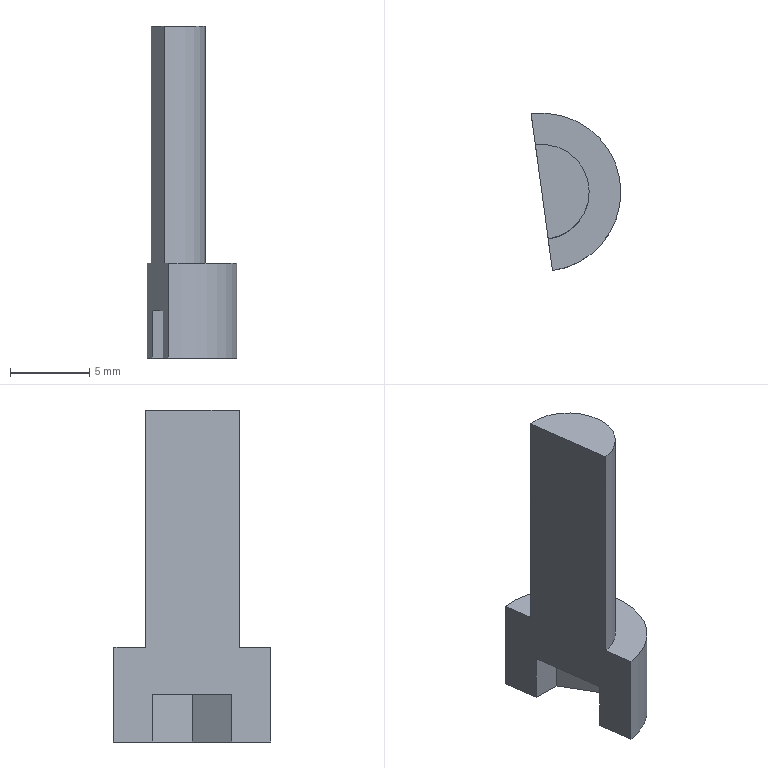Part | STEP file | LG M6_1.5F | 1 solid | 12 faces | box 5.673 x 9.954 x 21 mm | volume 414.941 mm3 | plane 9 | cylinder 3 | commonest cylinder face diameters 10 x2 6 x1
STEP:
#1=CARTESIAN_POINT('',(0.,0.,0.));
#2=DIRECTION('',(0.,0.,1.));
#3=DIRECTION('',(1.,0.,0.));
#4=AXIS2_PLACEMENT_3D('',#1,#2,#3);
#5=CARTESIAN_POINT('',(0.6731,-4.954,-6.));
#6=VERTEX_POINT('',#5);
#7=CARTESIAN_POINT('',(5.,0.,-6.));
#8=VERTEX_POINT('',#7);
#9=CARTESIAN_POINT('',(0.,0.,-6.));
#10=DIRECTION('',(0.,0.,1.));
#11=DIRECTION('',(1.,0.,0.));
#12=AXIS2_PLACEMENT_3D('',#9,#10,#11);
#13=CIRCLE('',#12,5.);
#14=CARTESIAN_POINT('',(0.,0.,-6.));
#15=DIRECTION('',(0.,0.,1.));
#16=DIRECTION('',(1.,0.,0.));
#17=AXIS2_PLACEMENT_3D('',#14,#15,#16);
#18=CYLINDRICAL_SURFACE('',#17,5.);
#19=CARTESIAN_POINT('',(0.,0.));
#20=DIRECTION('',(1.,0.));
#21=VECTOR('',#20,1.);
#22=LINE('',#19,#21);
#23=(GEOMETRIC_REPRESENTATION_CONTEXT(2)PARAMETRIC_REPRESENTATION_CONTEXT()REPRESENTATION_CONTEXT('',''));
#24=DEFINITIONAL_REPRESENTATION('',(#22),#23);
#25=PCURVE('',#18,#24);
#26=CARTESIAN_POINT('',(0.,0.,-6.));
#27=DIRECTION('',(0.,0.,1.));
#28=DIRECTION('',(1.,0.,0.));
#29=AXIS2_PLACEMENT_3D('',#26,#27,#28);
#30=PLANE('',#29);
#31=CARTESIAN_POINT('',(0.,0.));
#32=DIRECTION('',(1.,0.));
#33=AXIS2_PLACEMENT_2D('',#31,#32);
#34=CIRCLE('',#33,5.);
#35=(GEOMETRIC_REPRESENTATION_CONTEXT(2)PARAMETRIC_REPRESENTATION_CONTEXT()REPRESENTATION_CONTEXT('',''));
#36=DEFINITIONAL_REPRESENTATION('',(#34),#35);
#37=PCURVE('',#30,#36);
#38=SURFACE_CURVE('',#13,(#25,#37),.PCURVE_S1.);
#39=EDGE_CURVE('',#6,#8,#38,.T.);
#40=ORIENTED_EDGE('',*,*,#39,.T.);
#41=CARTESIAN_POINT('',(5.,0.,0.));
#42=VERTEX_POINT('',#41);
#43=CARTESIAN_POINT('',(5.,0.,-6.));
#44=DIRECTION('',(0.,0.,1.));
#45=VECTOR('',#44,1.);
#46=LINE('',#43,#45);
#47=CARTESIAN_POINT('',(6.283,0.));
#48=DIRECTION('',(0.,1.));
#49=VECTOR('',#48,1.);
#50=LINE('',#47,#49);
#51=(GEOMETRIC_REPRESENTATION_CONTEXT(2)PARAMETRIC_REPRESENTATION_CONTEXT()REPRESENTATION_CONTEXT('',''));
#52=DEFINITIONAL_REPRESENTATION('',(#50),#51);
#53=PCURVE('',#18,#52);
#54=CARTESIAN_POINT('',(0.,0.,-6.));
#55=DIRECTION('',(0.,0.,1.));
#56=DIRECTION('',(1.,0.,0.));
#57=AXIS2_PLACEMENT_3D('',#54,#55,#56);
#58=CYLINDRICAL_SURFACE('',#57,5.);
#59=CARTESIAN_POINT('',(0.,0.));
#60=DIRECTION('',(0.,1.));
#61=VECTOR('',#60,1.);
#62=LINE('',#59,#61);
#63=(GEOMETRIC_REPRESENTATION_CONTEXT(2)PARAMETRIC_REPRESENTATION_CONTEXT()REPRESENTATION_CONTEXT('',''));
#64=DEFINITIONAL_REPRESENTATION('',(#62),#63);
#65=PCURVE('',#58,#64);
#66=SURFACE_CURVE('',#46,(#53,#65),.PCURVE_S1.);
#67=EDGE_CURVE('',#8,#42,#66,.T.);
#68=ORIENTED_EDGE('',*,*,#67,.T.);
#69=CARTESIAN_POINT('',(0.6731,-4.954,0.));
#70=VERTEX_POINT('',#69);
#71=CARTESIAN_POINT('',(0.,0.,0.));
#72=DIRECTION('',(0.,0.,1.));
#73=DIRECTION('',(1.,0.,0.));
#74=AXIS2_PLACEMENT_3D('',#71,#72,#73);
#75=CIRCLE('',#74,5.);
#76=CARTESIAN_POINT('',(0.,6.));
#77=DIRECTION('',(1.,0.));
#78=VECTOR('',#77,1.);
#79=LINE('',#76,#78);
#80=(GEOMETRIC_REPRESENTATION_CONTEXT(2)PARAMETRIC_REPRESENTATION_CONTEXT()REPRESENTATION_CONTEXT('',''));
#81=DEFINITIONAL_REPRESENTATION('',(#79),#80);
#82=PCURVE('',#18,#81);
#83=CARTESIAN_POINT('',(0.,0.,0.));
#84=DIRECTION('',(0.,0.,1.));
#85=DIRECTION('',(1.,0.,0.));
#86=AXIS2_PLACEMENT_3D('',#83,#84,#85);
#87=PLANE('',#86);
#88=CARTESIAN_POINT('',(0.,0.));
#89=DIRECTION('',(1.,0.));
#90=AXIS2_PLACEMENT_2D('',#88,#89);
#91=CIRCLE('',#90,5.);
#92=(GEOMETRIC_REPRESENTATION_CONTEXT(2)PARAMETRIC_REPRESENTATION_CONTEXT()REPRESENTATION_CONTEXT('',''));
#93=DEFINITIONAL_REPRESENTATION('',(#91),#92);
#94=PCURVE('',#87,#93);
#95=SURFACE_CURVE('',#75,(#82,#94),.PCURVE_S1.);
#96=EDGE_CURVE('',#70,#42,#95,.T.);
#97=ORIENTED_EDGE('',*,*,#96,.F.);
#98=CARTESIAN_POINT('',(0.6731,-4.954,-6.));
#99=DIRECTION('',(0.,0.,1.));
#100=VECTOR('',#99,1.);
#101=LINE('',#98,#100);
#102=CARTESIAN_POINT('',(4.847,0.));
#103=DIRECTION('',(0.,1.));
#104=VECTOR('',#103,1.);
#105=LINE('',#102,#104);
#106=(GEOMETRIC_REPRESENTATION_CONTEXT(2)PARAMETRIC_REPRESENTATION_CONTEXT()REPRESENTATION_CONTEXT('',''));
#107=DEFINITIONAL_REPRESENTATION('',(#105),#106);
#108=PCURVE('',#18,#107);
#109=CARTESIAN_POINT('',(8.077,-59.454,72.57));
#110=DIRECTION('',(0.9909,0.1346,0.));
#111=DIRECTION('',(0.1346,-0.9909,0.));
#112=AXIS2_PLACEMENT_3D('',#109,#110,#111);
#113=PLANE('',#112);
#114=CARTESIAN_POINT('',(-55.,78.57));
#115=DIRECTION('',(0.,-1.));
#116=VECTOR('',#115,1.);
#117=LINE('',#114,#116);
#118=(GEOMETRIC_REPRESENTATION_CONTEXT(2)PARAMETRIC_REPRESENTATION_CONTEXT()REPRESENTATION_CONTEXT('',''));
#119=DEFINITIONAL_REPRESENTATION('',(#117),#118);
#120=PCURVE('',#113,#119);
#121=SURFACE_CURVE('',#101,(#108,#120),.PCURVE_S1.);
#122=EDGE_CURVE('',#6,#70,#121,.T.);
#123=ORIENTED_EDGE('',*,*,#122,.F.);
#124=EDGE_LOOP('',(#40,#68,#97,#123));
#125=FACE_BOUND('',#124,.T.);
#126=ADVANCED_FACE('',(#125),#18,.T.);
#127=CARTESIAN_POINT('',(0.4039,-2.973,0.));
#128=VERTEX_POINT('',#127);
#129=CARTESIAN_POINT('',(0.,0.,0.));
#130=DIRECTION('',(-0.1346,0.9909,0.));
#131=VECTOR('',#130,1.);
#132=LINE('',#129,#131);
#133=CARTESIAN_POINT('',(0.,0.));
#134=DIRECTION('',(-0.1346,0.9909));
#135=VECTOR('',#134,1.);
#136=LINE('',#133,#135);
#137=(GEOMETRIC_REPRESENTATION_CONTEXT(2)PARAMETRIC_REPRESENTATION_CONTEXT()REPRESENTATION_CONTEXT('',''));
#138=DEFINITIONAL_REPRESENTATION('',(#136),#137);
#139=PCURVE('',#87,#138);
#140=CARTESIAN_POINT('',(-60.,72.57));
#141=DIRECTION('',(-1.,0.));
#142=VECTOR('',#141,1.);
#143=LINE('',#140,#142);
#144=(GEOMETRIC_REPRESENTATION_CONTEXT(2)PARAMETRIC_REPRESENTATION_CONTEXT()REPRESENTATION_CONTEXT('',''));
#145=DEFINITIONAL_REPRESENTATION('',(#143),#144);
#146=PCURVE('',#113,#145);
#147=SURFACE_CURVE('',#132,(#139,#146),.PCURVE_S1.);
#148=EDGE_CURVE('',#70,#128,#147,.T.);
#149=ORIENTED_EDGE('',*,*,#148,.F.);
#150=ORIENTED_EDGE('',*,*,#96,.T.);
#151=CARTESIAN_POINT('',(-0.6731,4.954,0.));
#152=VERTEX_POINT('',#151);
#153=CARTESIAN_POINT('',(0.,0.,0.));
#154=DIRECTION('',(0.,0.,1.));
#155=DIRECTION('',(1.,0.,0.));
#156=AXIS2_PLACEMENT_3D('',#153,#154,#155);
#157=CIRCLE('',#156,5.);
#158=CARTESIAN_POINT('',(0.,0.));
#159=DIRECTION('',(1.,0.));
#160=AXIS2_PLACEMENT_2D('',#158,#159);
#161=CIRCLE('',#160,5.);
#162=(GEOMETRIC_REPRESENTATION_CONTEXT(2)PARAMETRIC_REPRESENTATION_CONTEXT()REPRESENTATION_CONTEXT('',''));
#163=DEFINITIONAL_REPRESENTATION('',(#161),#162);
#164=PCURVE('',#87,#163);
#165=CARTESIAN_POINT('',(0.,6.));
#166=DIRECTION('',(1.,0.));
#167=VECTOR('',#166,1.);
#168=LINE('',#165,#167);
#169=(GEOMETRIC_REPRESENTATION_CONTEXT(2)PARAMETRIC_REPRESENTATION_CONTEXT()REPRESENTATION_CONTEXT('',''));
#170=DEFINITIONAL_REPRESENTATION('',(#168),#169);
#171=PCURVE('',#58,#170);
#172=SURFACE_CURVE('',#157,(#164,#171),.PCURVE_S1.);
#173=EDGE_CURVE('',#42,#152,#172,.T.);
#174=ORIENTED_EDGE('',*,*,#173,.T.);
#175=CARTESIAN_POINT('',(-0.4039,2.973,0.));
#176=VERTEX_POINT('',#175);
#177=CARTESIAN_POINT('',(0.,0.,0.));
#178=DIRECTION('',(-0.1346,0.9909,0.));
#179=VECTOR('',#178,1.);
#180=LINE('',#177,#179);
#181=CARTESIAN_POINT('',(0.,0.));
#182=DIRECTION('',(-0.1346,0.9909));
#183=VECTOR('',#182,1.);
#184=LINE('',#181,#183);
#185=(GEOMETRIC_REPRESENTATION_CONTEXT(2)PARAMETRIC_REPRESENTATION_CONTEXT()REPRESENTATION_CONTEXT('',''));
#186=DEFINITIONAL_REPRESENTATION('',(#184),#185);
#187=PCURVE('',#87,#186);
#188=CARTESIAN_POINT('',(-60.,72.57));
#189=DIRECTION('',(-1.,0.));
#190=VECTOR('',#189,1.);
#191=LINE('',#188,#190);
#192=(GEOMETRIC_REPRESENTATION_CONTEXT(2)PARAMETRIC_REPRESENTATION_CONTEXT()REPRESENTATION_CONTEXT('',''));
#193=DEFINITIONAL_REPRESENTATION('',(#191),#192);
#194=PCURVE('',#113,#193);
#195=SURFACE_CURVE('',#180,(#187,#194),.PCURVE_S1.);
#196=EDGE_CURVE('',#176,#152,#195,.T.);
#197=ORIENTED_EDGE('',*,*,#196,.F.);
#198=CARTESIAN_POINT('',(0.,0.,0.));
#199=DIRECTION('',(0.,0.,1.));
#200=DIRECTION('',(1.,0.,0.));
#201=AXIS2_PLACEMENT_3D('',#198,#199,#200);
#202=CIRCLE('',#201,3.);
#203=CARTESIAN_POINT('',(0.,0.));
#204=DIRECTION('',(1.,0.));
#205=AXIS2_PLACEMENT_2D('',#203,#204);
#206=CIRCLE('',#205,3.);
#207=(GEOMETRIC_REPRESENTATION_CONTEXT(2)PARAMETRIC_REPRESENTATION_CONTEXT()REPRESENTATION_CONTEXT('',''));
#208=DEFINITIONAL_REPRESENTATION('',(#206),#207);
#209=PCURVE('',#87,#208);
#210=CARTESIAN_POINT('',(0.,0.,15.));
#211=DIRECTION('',(0.,0.,-1.));
#212=DIRECTION('',(-1.,0.,0.));
#213=AXIS2_PLACEMENT_3D('',#210,#211,#212);
#214=CYLINDRICAL_SURFACE('',#213,3.);
#215=CARTESIAN_POINT('',(9.425,15.));
#216=DIRECTION('',(-1.,0.));
#217=VECTOR('',#216,1.);
#218=LINE('',#215,#217);
#219=(GEOMETRIC_REPRESENTATION_CONTEXT(2)PARAMETRIC_REPRESENTATION_CONTEXT()REPRESENTATION_CONTEXT('',''));
#220=DEFINITIONAL_REPRESENTATION('',(#218),#219);
#221=PCURVE('',#214,#220);
#222=SURFACE_CURVE('',#202,(#209,#221),.PCURVE_S1.);
#223=EDGE_CURVE('',#128,#176,#222,.T.);
#224=ORIENTED_EDGE('',*,*,#223,.F.);
#225=EDGE_LOOP('',(#149,#150,#174,#197,#224));
#226=FACE_BOUND('',#225,.T.);
#227=ADVANCED_FACE('',(#226),#87,.T.);
#228=ORIENTED_EDGE('',*,*,#67,.F.);
#229=CARTESIAN_POINT('',(-0.6731,4.954,-6.));
#230=VERTEX_POINT('',#229);
#231=CARTESIAN_POINT('',(0.,0.,-6.));
#232=DIRECTION('',(0.,0.,1.));
#233=DIRECTION('',(1.,0.,0.));
#234=AXIS2_PLACEMENT_3D('',#231,#232,#233);
#235=CIRCLE('',#234,5.);
#236=CARTESIAN_POINT('',(0.,0.));
#237=DIRECTION('',(1.,0.));
#238=VECTOR('',#237,1.);
#239=LINE('',#236,#238);
#240=(GEOMETRIC_REPRESENTATION_CONTEXT(2)PARAMETRIC_REPRESENTATION_CONTEXT()REPRESENTATION_CONTEXT('',''));
#241=DEFINITIONAL_REPRESENTATION('',(#239),#240);
#242=PCURVE('',#58,#241);
#243=CARTESIAN_POINT('',(0.,0.));
#244=DIRECTION('',(1.,0.));
#245=AXIS2_PLACEMENT_2D('',#243,#244);
#246=CIRCLE('',#245,5.);
#247=(GEOMETRIC_REPRESENTATION_CONTEXT(2)PARAMETRIC_REPRESENTATION_CONTEXT()REPRESENTATION_CONTEXT('',''));
#248=DEFINITIONAL_REPRESENTATION('',(#246),#247);
#249=PCURVE('',#30,#248);
#250=SURFACE_CURVE('',#235,(#242,#249),.PCURVE_S1.);
#251=EDGE_CURVE('',#8,#230,#250,.T.);
#252=ORIENTED_EDGE('',*,*,#251,.T.);
#253=CARTESIAN_POINT('',(-0.6731,4.954,-6.));
#254=DIRECTION('',(0.,0.,-1.));
#255=VECTOR('',#254,1.);
#256=LINE('',#253,#255);
#257=CARTESIAN_POINT('',(1.706,0.));
#258=DIRECTION('',(0.,-1.));
#259=VECTOR('',#258,1.);
#260=LINE('',#257,#259);
#261=(GEOMETRIC_REPRESENTATION_CONTEXT(2)PARAMETRIC_REPRESENTATION_CONTEXT()REPRESENTATION_CONTEXT('',''));
#262=DEFINITIONAL_REPRESENTATION('',(#260),#261);
#263=PCURVE('',#58,#262);
#264=CARTESIAN_POINT('',(-65.,78.57));
#265=DIRECTION('',(0.,1.));
#266=VECTOR('',#265,1.);
#267=LINE('',#264,#266);
#268=(GEOMETRIC_REPRESENTATION_CONTEXT(2)PARAMETRIC_REPRESENTATION_CONTEXT()REPRESENTATION_CONTEXT('',''));
#269=DEFINITIONAL_REPRESENTATION('',(#267),#268);
#270=PCURVE('',#113,#269);
#271=SURFACE_CURVE('',#256,(#263,#270),.PCURVE_S1.);
#272=EDGE_CURVE('',#152,#230,#271,.T.);
#273=ORIENTED_EDGE('',*,*,#272,.F.);
#274=ORIENTED_EDGE('',*,*,#173,.F.);
#275=EDGE_LOOP('',(#228,#252,#273,#274));
#276=FACE_BOUND('',#275,.T.);
#277=ADVANCED_FACE('',(#276),#58,.T.);
#278=ORIENTED_EDGE('',*,*,#39,.F.);
#279=CARTESIAN_POINT('',(0.341,-2.51,-6.));
#280=VERTEX_POINT('',#279);
#281=CARTESIAN_POINT('',(0.,0.,-6.));
#282=DIRECTION('',(-0.1346,0.9909,0.));
#283=VECTOR('',#282,1.);
#284=LINE('',#281,#283);
#285=CARTESIAN_POINT('',(0.,0.));
#286=DIRECTION('',(-0.1346,0.9909));
#287=VECTOR('',#286,1.);
#288=LINE('',#285,#287);
#289=(GEOMETRIC_REPRESENTATION_CONTEXT(2)PARAMETRIC_REPRESENTATION_CONTEXT()REPRESENTATION_CONTEXT('',''));
#290=DEFINITIONAL_REPRESENTATION('',(#288),#289);
#291=PCURVE('',#30,#290);
#292=CARTESIAN_POINT('',(-60.,78.57));
#293=DIRECTION('',(-1.,0.));
#294=VECTOR('',#293,1.);
#295=LINE('',#292,#294);
#296=(GEOMETRIC_REPRESENTATION_CONTEXT(2)PARAMETRIC_REPRESENTATION_CONTEXT()REPRESENTATION_CONTEXT('',''));
#297=DEFINITIONAL_REPRESENTATION('',(#295),#296);
#298=PCURVE('',#113,#297);
#299=SURFACE_CURVE('',#284,(#291,#298),.PCURVE_S1.);
#300=EDGE_CURVE('',#6,#280,#299,.T.);
#301=ORIENTED_EDGE('',*,*,#300,.T.);
#302=CARTESIAN_POINT('',(1.449,-2.51,-6.));
#303=VERTEX_POINT('',#302);
#304=CARTESIAN_POINT('',(1.449,-2.51,-6.));
#305=DIRECTION('',(-1.,0.,0.));
#306=VECTOR('',#305,1.);
#307=LINE('',#304,#306);
#308=CARTESIAN_POINT('',(1.449,-2.51));
#309=DIRECTION('',(-1.,0.));
#310=VECTOR('',#309,1.);
#311=LINE('',#308,#310);
#312=(GEOMETRIC_REPRESENTATION_CONTEXT(2)PARAMETRIC_REPRESENTATION_CONTEXT()REPRESENTATION_CONTEXT('',''));
#313=DEFINITIONAL_REPRESENTATION('',(#311),#312);
#314=PCURVE('',#30,#313);
#315=CARTESIAN_POINT('',(1.449,-2.51,-3.));
#316=DIRECTION('',(0.,-1.,0.));
#317=DIRECTION('',(0.,0.,-1.));
#318=AXIS2_PLACEMENT_3D('',#315,#316,#317);
#319=PLANE('',#318);
#320=CARTESIAN_POINT('',(3.,0.));
#321=DIRECTION('',(0.,-1.));
#322=VECTOR('',#321,1.);
#323=LINE('',#320,#322);
#324=(GEOMETRIC_REPRESENTATION_CONTEXT(2)PARAMETRIC_REPRESENTATION_CONTEXT()REPRESENTATION_CONTEXT('',''));
#325=DEFINITIONAL_REPRESENTATION('',(#323),#324);
#326=PCURVE('',#319,#325);
#327=SURFACE_CURVE('',#307,(#314,#326),.PCURVE_S1.);
#328=EDGE_CURVE('',#303,#280,#327,.T.);
#329=ORIENTED_EDGE('',*,*,#328,.F.);
#330=CARTESIAN_POINT('',(2.898,0.,-6.));
#331=VERTEX_POINT('',#330);
#332=CARTESIAN_POINT('',(2.898,0.,-6.));
#333=DIRECTION('',(-0.5,-0.866,0.));
#334=VECTOR('',#333,1.);
#335=LINE('',#332,#334);
#336=CARTESIAN_POINT('',(2.898,0.));
#337=DIRECTION('',(-0.5,-0.866));
#338=VECTOR('',#337,1.);
#339=LINE('',#336,#338);
#340=(GEOMETRIC_REPRESENTATION_CONTEXT(2)PARAMETRIC_REPRESENTATION_CONTEXT()REPRESENTATION_CONTEXT('',''));
#341=DEFINITIONAL_REPRESENTATION('',(#339),#340);
#342=PCURVE('',#30,#341);
#343=CARTESIAN_POINT('',(2.898,0.,-3.));
#344=DIRECTION('',(0.866,-0.5,0.));
#345=DIRECTION('',(0.5,0.866,0.));
#346=AXIS2_PLACEMENT_3D('',#343,#344,#345);
#347=PLANE('',#346);
#348=CARTESIAN_POINT('',(0.,-3.));
#349=DIRECTION('',(-1.,0.));
#350=VECTOR('',#349,1.);
#351=LINE('',#348,#350);
#352=(GEOMETRIC_REPRESENTATION_CONTEXT(2)PARAMETRIC_REPRESENTATION_CONTEXT()REPRESENTATION_CONTEXT('',''));
#353=DEFINITIONAL_REPRESENTATION('',(#351),#352);
#354=PCURVE('',#347,#353);
#355=SURFACE_CURVE('',#335,(#342,#354),.PCURVE_S1.);
#356=EDGE_CURVE('',#331,#303,#355,.T.);
#357=ORIENTED_EDGE('',*,*,#356,.F.);
#358=CARTESIAN_POINT('',(1.449,2.51,-6.));
#359=VERTEX_POINT('',#358);
#360=CARTESIAN_POINT('',(1.449,2.51,-6.));
#361=DIRECTION('',(0.5,-0.866,0.));
#362=VECTOR('',#361,1.);
#363=LINE('',#360,#362);
#364=CARTESIAN_POINT('',(1.449,2.51));
#365=DIRECTION('',(0.5,-0.866));
#366=VECTOR('',#365,1.);
#367=LINE('',#364,#366);
#368=(GEOMETRIC_REPRESENTATION_CONTEXT(2)PARAMETRIC_REPRESENTATION_CONTEXT()REPRESENTATION_CONTEXT('',''));
#369=DEFINITIONAL_REPRESENTATION('',(#367),#368);
#370=PCURVE('',#30,#369);
#371=CARTESIAN_POINT('',(1.449,2.51,-3.));
#372=DIRECTION('',(0.866,0.5,0.));
#373=DIRECTION('',(-0.5,0.866,0.));
#374=AXIS2_PLACEMENT_3D('',#371,#372,#373);
#375=PLANE('',#374);
#376=CARTESIAN_POINT('',(0.,-3.));
#377=DIRECTION('',(-1.,0.));
#378=VECTOR('',#377,1.);
#379=LINE('',#376,#378);
#380=(GEOMETRIC_REPRESENTATION_CONTEXT(2)PARAMETRIC_REPRESENTATION_CONTEXT()REPRESENTATION_CONTEXT('',''));
#381=DEFINITIONAL_REPRESENTATION('',(#379),#380);
#382=PCURVE('',#375,#381);
#383=SURFACE_CURVE('',#363,(#370,#382),.PCURVE_S1.);
#384=EDGE_CURVE('',#359,#331,#383,.T.);
#385=ORIENTED_EDGE('',*,*,#384,.F.);
#386=CARTESIAN_POINT('',(-0.341,2.51,-6.));
#387=VERTEX_POINT('',#386);
#388=CARTESIAN_POINT('',(-1.449,2.51,-6.));
#389=DIRECTION('',(1.,0.,0.));
#390=VECTOR('',#389,1.);
#391=LINE('',#388,#390);
#392=CARTESIAN_POINT('',(-1.449,2.51));
#393=DIRECTION('',(1.,0.));
#394=VECTOR('',#393,1.);
#395=LINE('',#392,#394);
#396=(GEOMETRIC_REPRESENTATION_CONTEXT(2)PARAMETRIC_REPRESENTATION_CONTEXT()REPRESENTATION_CONTEXT('',''));
#397=DEFINITIONAL_REPRESENTATION('',(#395),#396);
#398=PCURVE('',#30,#397);
#399=CARTESIAN_POINT('',(-1.449,2.51,-3.));
#400=DIRECTION('',(0.,1.,0.));
#401=DIRECTION('',(0.,0.,1.));
#402=AXIS2_PLACEMENT_3D('',#399,#400,#401);
#403=PLANE('',#402);
#404=CARTESIAN_POINT('',(-3.,0.));
#405=DIRECTION('',(0.,1.));
#406=VECTOR('',#405,1.);
#407=LINE('',#404,#406);
#408=(GEOMETRIC_REPRESENTATION_CONTEXT(2)PARAMETRIC_REPRESENTATION_CONTEXT()REPRESENTATION_CONTEXT('',''));
#409=DEFINITIONAL_REPRESENTATION('',(#407),#408);
#410=PCURVE('',#403,#409);
#411=SURFACE_CURVE('',#391,(#398,#410),.PCURVE_S1.);
#412=EDGE_CURVE('',#387,#359,#411,.T.);
#413=ORIENTED_EDGE('',*,*,#412,.F.);
#414=CARTESIAN_POINT('',(0.,0.,-6.));
#415=DIRECTION('',(-0.1346,0.9909,0.));
#416=VECTOR('',#415,1.);
#417=LINE('',#414,#416);
#418=CARTESIAN_POINT('',(0.,0.));
#419=DIRECTION('',(-0.1346,0.9909));
#420=VECTOR('',#419,1.);
#421=LINE('',#418,#420);
#422=(GEOMETRIC_REPRESENTATION_CONTEXT(2)PARAMETRIC_REPRESENTATION_CONTEXT()REPRESENTATION_CONTEXT('',''));
#423=DEFINITIONAL_REPRESENTATION('',(#421),#422);
#424=PCURVE('',#30,#423);
#425=CARTESIAN_POINT('',(-60.,78.57));
#426=DIRECTION('',(-1.,0.));
#427=VECTOR('',#426,1.);
#428=LINE('',#425,#427);
#429=(GEOMETRIC_REPRESENTATION_CONTEXT(2)PARAMETRIC_REPRESENTATION_CONTEXT()REPRESENTATION_CONTEXT('',''));
#430=DEFINITIONAL_REPRESENTATION('',(#428),#429);
#431=PCURVE('',#113,#430);
#432=SURFACE_CURVE('',#417,(#424,#431),.PCURVE_S1.);
#433=EDGE_CURVE('',#387,#230,#432,.T.);
#434=ORIENTED_EDGE('',*,*,#433,.T.);
#435=ORIENTED_EDGE('',*,*,#251,.F.);
#436=EDGE_LOOP('',(#278,#301,#329,#357,#385,#413,#434,#435));
#437=FACE_BOUND('',#436,.T.);
#438=ADVANCED_FACE('',(#437),#30,.F.);
#439=CARTESIAN_POINT('',(0.4039,-2.973,15.));
#440=VERTEX_POINT('',#439);
#441=CARTESIAN_POINT('',(-0.4039,2.973,15.));
#442=VERTEX_POINT('',#441);
#443=CARTESIAN_POINT('',(0.,0.,15.));
#444=DIRECTION('',(0.,0.,1.));
#445=DIRECTION('',(1.,0.,0.));
#446=AXIS2_PLACEMENT_3D('',#443,#444,#445);
#447=CIRCLE('',#446,3.);
#448=CARTESIAN_POINT('',(9.425,0.));
#449=DIRECTION('',(-1.,0.));
#450=VECTOR('',#449,1.);
#451=LINE('',#448,#450);
#452=(GEOMETRIC_REPRESENTATION_CONTEXT(2)PARAMETRIC_REPRESENTATION_CONTEXT()REPRESENTATION_CONTEXT('',''));
#453=DEFINITIONAL_REPRESENTATION('',(#451),#452);
#454=PCURVE('',#214,#453);
#455=CARTESIAN_POINT('',(0.,0.,15.));
#456=DIRECTION('',(0.,0.,1.));
#457=DIRECTION('',(1.,0.,0.));
#458=AXIS2_PLACEMENT_3D('',#455,#456,#457);
#459=PLANE('',#458);
#460=CARTESIAN_POINT('',(0.,0.));
#461=DIRECTION('',(1.,0.));
#462=AXIS2_PLACEMENT_2D('',#460,#461);
#463=CIRCLE('',#462,3.);
#464=(GEOMETRIC_REPRESENTATION_CONTEXT(2)PARAMETRIC_REPRESENTATION_CONTEXT()REPRESENTATION_CONTEXT('',''));
#465=DEFINITIONAL_REPRESENTATION('',(#463),#464);
#466=PCURVE('',#459,#465);
#467=SURFACE_CURVE('',#447,(#454,#466),.PCURVE_S1.);
#468=EDGE_CURVE('',#440,#442,#467,.T.);
#469=ORIENTED_EDGE('',*,*,#468,.F.);
#470=CARTESIAN_POINT('',(0.4039,-2.973,15.));
#471=DIRECTION('',(0.,0.,-1.));
#472=VECTOR('',#471,1.);
#473=LINE('',#470,#472);
#474=CARTESIAN_POINT('',(4.577,0.));
#475=DIRECTION('',(0.,1.));
#476=VECTOR('',#475,1.);
#477=LINE('',#474,#476);
#478=(GEOMETRIC_REPRESENTATION_CONTEXT(2)PARAMETRIC_REPRESENTATION_CONTEXT()REPRESENTATION_CONTEXT('',''));
#479=DEFINITIONAL_REPRESENTATION('',(#477),#478);
#480=PCURVE('',#214,#479);
#481=CARTESIAN_POINT('',(-57.,57.57));
#482=DIRECTION('',(0.,1.));
#483=VECTOR('',#482,1.);
#484=LINE('',#481,#483);
#485=(GEOMETRIC_REPRESENTATION_CONTEXT(2)PARAMETRIC_REPRESENTATION_CONTEXT()REPRESENTATION_CONTEXT('',''));
#486=DEFINITIONAL_REPRESENTATION('',(#484),#485);
#487=PCURVE('',#113,#486);
#488=SURFACE_CURVE('',#473,(#480,#487),.PCURVE_S1.);
#489=EDGE_CURVE('',#440,#128,#488,.T.);
#490=ORIENTED_EDGE('',*,*,#489,.T.);
#491=ORIENTED_EDGE('',*,*,#223,.T.);
#492=CARTESIAN_POINT('',(-0.4039,2.973,15.));
#493=DIRECTION('',(0.,0.,1.));
#494=VECTOR('',#493,1.);
#495=LINE('',#492,#494);
#496=CARTESIAN_POINT('',(1.436,0.));
#497=DIRECTION('',(0.,-1.));
#498=VECTOR('',#497,1.);
#499=LINE('',#496,#498);
#500=(GEOMETRIC_REPRESENTATION_CONTEXT(2)PARAMETRIC_REPRESENTATION_CONTEXT()REPRESENTATION_CONTEXT('',''));
#501=DEFINITIONAL_REPRESENTATION('',(#499),#500);
#502=PCURVE('',#214,#501);
#503=CARTESIAN_POINT('',(-63.,57.57));
#504=DIRECTION('',(0.,-1.));
#505=VECTOR('',#504,1.);
#506=LINE('',#503,#505);
#507=(GEOMETRIC_REPRESENTATION_CONTEXT(2)PARAMETRIC_REPRESENTATION_CONTEXT()REPRESENTATION_CONTEXT('',''));
#508=DEFINITIONAL_REPRESENTATION('',(#506),#507);
#509=PCURVE('',#113,#508);
#510=SURFACE_CURVE('',#495,(#502,#509),.PCURVE_S1.);
#511=EDGE_CURVE('',#176,#442,#510,.T.);
#512=ORIENTED_EDGE('',*,*,#511,.T.);
#513=EDGE_LOOP('',(#469,#490,#491,#512));
#514=FACE_BOUND('',#513,.T.);
#515=ADVANCED_FACE('',(#514),#214,.T.);
#516=CARTESIAN_POINT('',(0.,0.,15.));
#517=DIRECTION('',(-0.1346,0.9909,0.));
#518=VECTOR('',#517,1.);
#519=LINE('',#516,#518);
#520=CARTESIAN_POINT('',(0.,0.));
#521=DIRECTION('',(-0.1346,0.9909));
#522=VECTOR('',#521,1.);
#523=LINE('',#520,#522);
#524=(GEOMETRIC_REPRESENTATION_CONTEXT(2)PARAMETRIC_REPRESENTATION_CONTEXT()REPRESENTATION_CONTEXT('',''));
#525=DEFINITIONAL_REPRESENTATION('',(#523),#524);
#526=PCURVE('',#459,#525);
#527=CARTESIAN_POINT('',(-60.,57.57));
#528=DIRECTION('',(-1.,0.));
#529=VECTOR('',#528,1.);
#530=LINE('',#527,#529);
#531=(GEOMETRIC_REPRESENTATION_CONTEXT(2)PARAMETRIC_REPRESENTATION_CONTEXT()REPRESENTATION_CONTEXT('',''));
#532=DEFINITIONAL_REPRESENTATION('',(#530),#531);
#533=PCURVE('',#113,#532);
#534=SURFACE_CURVE('',#519,(#526,#533),.PCURVE_S1.);
#535=EDGE_CURVE('',#440,#442,#534,.T.);
#536=ORIENTED_EDGE('',*,*,#535,.F.);
#537=ORIENTED_EDGE('',*,*,#468,.T.);
#538=EDGE_LOOP('',(#536,#537));
#539=FACE_BOUND('',#538,.T.);
#540=ADVANCED_FACE('',(#539),#459,.T.);
#541=ORIENTED_EDGE('',*,*,#328,.T.);
#542=CARTESIAN_POINT('',(0.341,-2.51,-3.));
#543=VERTEX_POINT('',#542);
#544=CARTESIAN_POINT('',(0.341,-2.51,-3.));
#545=DIRECTION('',(0.,0.,1.));
#546=VECTOR('',#545,1.);
#547=LINE('',#544,#546);
#548=CARTESIAN_POINT('',(0.,-1.108));
#549=DIRECTION('',(-1.,0.));
#550=VECTOR('',#549,1.);
#551=LINE('',#548,#550);
#552=(GEOMETRIC_REPRESENTATION_CONTEXT(2)PARAMETRIC_REPRESENTATION_CONTEXT()REPRESENTATION_CONTEXT('',''));
#553=DEFINITIONAL_REPRESENTATION('',(#551),#552);
#554=PCURVE('',#319,#553);
#555=CARTESIAN_POINT('',(-57.467,75.57));
#556=DIRECTION('',(0.,-1.));
#557=VECTOR('',#556,1.);
#558=LINE('',#555,#557);
#559=(GEOMETRIC_REPRESENTATION_CONTEXT(2)PARAMETRIC_REPRESENTATION_CONTEXT()REPRESENTATION_CONTEXT('',''));
#560=DEFINITIONAL_REPRESENTATION('',(#558),#559);
#561=PCURVE('',#113,#560);
#562=SURFACE_CURVE('',#547,(#554,#561),.PCURVE_S1.);
#563=EDGE_CURVE('',#280,#543,#562,.T.);
#564=ORIENTED_EDGE('',*,*,#563,.T.);
#565=CARTESIAN_POINT('',(1.449,-2.51,-3.));
#566=VERTEX_POINT('',#565);
#567=CARTESIAN_POINT('',(1.449,-2.51,-3.));
#568=DIRECTION('',(-1.,0.,0.));
#569=VECTOR('',#568,1.);
#570=LINE('',#567,#569);
#571=CARTESIAN_POINT('',(0.,0.));
#572=DIRECTION('',(0.,-1.));
#573=VECTOR('',#572,1.);
#574=LINE('',#571,#573);
#575=(GEOMETRIC_REPRESENTATION_CONTEXT(2)PARAMETRIC_REPRESENTATION_CONTEXT()REPRESENTATION_CONTEXT('',''));
#576=DEFINITIONAL_REPRESENTATION('',(#574),#575);
#577=PCURVE('',#319,#576);
#578=CARTESIAN_POINT('',(0.,0.,-3.));
#579=DIRECTION('',(0.,0.,-1.));
#580=DIRECTION('',(-1.,0.,0.));
#581=AXIS2_PLACEMENT_3D('',#578,#579,#580);
#582=PLANE('',#581);
#583=CARTESIAN_POINT('',(-1.449,-2.51));
#584=DIRECTION('',(1.,0.));
#585=VECTOR('',#584,1.);
#586=LINE('',#583,#585);
#587=(GEOMETRIC_REPRESENTATION_CONTEXT(2)PARAMETRIC_REPRESENTATION_CONTEXT()REPRESENTATION_CONTEXT('',''));
#588=DEFINITIONAL_REPRESENTATION('',(#586),#587);
#589=PCURVE('',#582,#588);
#590=SURFACE_CURVE('',#570,(#577,#589),.PCURVE_S1.);
#591=EDGE_CURVE('',#566,#543,#590,.T.);
#592=ORIENTED_EDGE('',*,*,#591,.F.);
#593=CARTESIAN_POINT('',(1.449,-2.51,-3.));
#594=DIRECTION('',(0.,0.,-1.));
#595=VECTOR('',#594,1.);
#596=LINE('',#593,#595);
#597=CARTESIAN_POINT('',(0.,0.));
#598=DIRECTION('',(1.,0.));
#599=VECTOR('',#598,1.);
#600=LINE('',#597,#599);
#601=(GEOMETRIC_REPRESENTATION_CONTEXT(2)PARAMETRIC_REPRESENTATION_CONTEXT()REPRESENTATION_CONTEXT('',''));
#602=DEFINITIONAL_REPRESENTATION('',(#600),#601);
#603=PCURVE('',#319,#602);
#604=CARTESIAN_POINT('',(-2.898,0.));
#605=DIRECTION('',(0.,-1.));
#606=VECTOR('',#605,1.);
#607=LINE('',#604,#606);
#608=(GEOMETRIC_REPRESENTATION_CONTEXT(2)PARAMETRIC_REPRESENTATION_CONTEXT()REPRESENTATION_CONTEXT('',''));
#609=DEFINITIONAL_REPRESENTATION('',(#607),#608);
#610=PCURVE('',#347,#609);
#611=SURFACE_CURVE('',#596,(#603,#610),.PCURVE_S1.);
#612=EDGE_CURVE('',#566,#303,#611,.T.);
#613=ORIENTED_EDGE('',*,*,#612,.T.);
#614=EDGE_LOOP('',(#541,#564,#592,#613));
#615=FACE_BOUND('',#614,.T.);
#616=ADVANCED_FACE('',(#615),#319,.F.);
#617=ORIENTED_EDGE('',*,*,#356,.T.);
#618=ORIENTED_EDGE('',*,*,#612,.F.);
#619=CARTESIAN_POINT('',(2.898,0.,-3.));
#620=VERTEX_POINT('',#619);
#621=CARTESIAN_POINT('',(2.898,0.,-3.));
#622=DIRECTION('',(-0.5,-0.866,0.));
#623=VECTOR('',#622,1.);
#624=LINE('',#621,#623);
#625=CARTESIAN_POINT('',(0.,0.));
#626=DIRECTION('',(-1.,0.));
#627=VECTOR('',#626,1.);
#628=LINE('',#625,#627);
#629=(GEOMETRIC_REPRESENTATION_CONTEXT(2)PARAMETRIC_REPRESENTATION_CONTEXT()REPRESENTATION_CONTEXT('',''));
#630=DEFINITIONAL_REPRESENTATION('',(#628),#629);
#631=PCURVE('',#347,#630);
#632=CARTESIAN_POINT('',(-2.898,0.));
#633=DIRECTION('',(0.5,-0.866));
#634=VECTOR('',#633,1.);
#635=LINE('',#632,#634);
#636=(GEOMETRIC_REPRESENTATION_CONTEXT(2)PARAMETRIC_REPRESENTATION_CONTEXT()REPRESENTATION_CONTEXT('',''));
#637=DEFINITIONAL_REPRESENTATION('',(#635),#636);
#638=PCURVE('',#582,#637);
#639=SURFACE_CURVE('',#624,(#631,#638),.PCURVE_S1.);
#640=EDGE_CURVE('',#620,#566,#639,.T.);
#641=ORIENTED_EDGE('',*,*,#640,.F.);
#642=CARTESIAN_POINT('',(2.898,0.,-3.));
#643=DIRECTION('',(0.,0.,-1.));
#644=VECTOR('',#643,1.);
#645=LINE('',#642,#644);
#646=CARTESIAN_POINT('',(0.,0.));
#647=DIRECTION('',(0.,-1.));
#648=VECTOR('',#647,1.);
#649=LINE('',#646,#648);
#650=(GEOMETRIC_REPRESENTATION_CONTEXT(2)PARAMETRIC_REPRESENTATION_CONTEXT()REPRESENTATION_CONTEXT('',''));
#651=DEFINITIONAL_REPRESENTATION('',(#649),#650);
#652=PCURVE('',#347,#651);
#653=CARTESIAN_POINT('',(-2.898,0.));
#654=DIRECTION('',(0.,-1.));
#655=VECTOR('',#654,1.);
#656=LINE('',#653,#655);
#657=(GEOMETRIC_REPRESENTATION_CONTEXT(2)PARAMETRIC_REPRESENTATION_CONTEXT()REPRESENTATION_CONTEXT('',''));
#658=DEFINITIONAL_REPRESENTATION('',(#656),#657);
#659=PCURVE('',#375,#658);
#660=SURFACE_CURVE('',#645,(#652,#659),.PCURVE_S1.);
#661=EDGE_CURVE('',#620,#331,#660,.T.);
#662=ORIENTED_EDGE('',*,*,#661,.T.);
#663=EDGE_LOOP('',(#617,#618,#641,#662));
#664=FACE_BOUND('',#663,.T.);
#665=ADVANCED_FACE('',(#664),#347,.F.);
#666=ORIENTED_EDGE('',*,*,#384,.T.);
#667=ORIENTED_EDGE('',*,*,#661,.F.);
#668=CARTESIAN_POINT('',(1.449,2.51,-3.));
#669=VERTEX_POINT('',#668);
#670=CARTESIAN_POINT('',(1.449,2.51,-3.));
#671=DIRECTION('',(0.5,-0.866,0.));
#672=VECTOR('',#671,1.);
#673=LINE('',#670,#672);
#674=CARTESIAN_POINT('',(0.,0.));
#675=DIRECTION('',(-1.,0.));
#676=VECTOR('',#675,1.);
#677=LINE('',#674,#676);
#678=(GEOMETRIC_REPRESENTATION_CONTEXT(2)PARAMETRIC_REPRESENTATION_CONTEXT()REPRESENTATION_CONTEXT('',''));
#679=DEFINITIONAL_REPRESENTATION('',(#677),#678);
#680=PCURVE('',#375,#679);
#681=CARTESIAN_POINT('',(-1.449,2.51));
#682=DIRECTION('',(-0.5,-0.866));
#683=VECTOR('',#682,1.);
#684=LINE('',#681,#683);
#685=(GEOMETRIC_REPRESENTATION_CONTEXT(2)PARAMETRIC_REPRESENTATION_CONTEXT()REPRESENTATION_CONTEXT('',''));
#686=DEFINITIONAL_REPRESENTATION('',(#684),#685);
#687=PCURVE('',#582,#686);
#688=SURFACE_CURVE('',#673,(#680,#687),.PCURVE_S1.);
#689=EDGE_CURVE('',#669,#620,#688,.T.);
#690=ORIENTED_EDGE('',*,*,#689,.F.);
#691=CARTESIAN_POINT('',(1.449,2.51,-3.));
#692=DIRECTION('',(0.,0.,-1.));
#693=VECTOR('',#692,1.);
#694=LINE('',#691,#693);
#695=CARTESIAN_POINT('',(0.,0.));
#696=DIRECTION('',(0.,-1.));
#697=VECTOR('',#696,1.);
#698=LINE('',#695,#697);
#699=(GEOMETRIC_REPRESENTATION_CONTEXT(2)PARAMETRIC_REPRESENTATION_CONTEXT()REPRESENTATION_CONTEXT('',''));
#700=DEFINITIONAL_REPRESENTATION('',(#698),#699);
#701=PCURVE('',#375,#700);
#702=CARTESIAN_POINT('',(0.,2.898));
#703=DIRECTION('',(-1.,0.));
#704=VECTOR('',#703,1.);
#705=LINE('',#702,#704);
#706=(GEOMETRIC_REPRESENTATION_CONTEXT(2)PARAMETRIC_REPRESENTATION_CONTEXT()REPRESENTATION_CONTEXT('',''));
#707=DEFINITIONAL_REPRESENTATION('',(#705),#706);
#708=PCURVE('',#403,#707);
#709=SURFACE_CURVE('',#694,(#701,#708),.PCURVE_S1.);
#710=EDGE_CURVE('',#669,#359,#709,.T.);
#711=ORIENTED_EDGE('',*,*,#710,.T.);
#712=EDGE_LOOP('',(#666,#667,#690,#711));
#713=FACE_BOUND('',#712,.T.);
#714=ADVANCED_FACE('',(#713),#375,.F.);
#715=CARTESIAN_POINT('',(-0.341,2.51,-3.));
#716=VERTEX_POINT('',#715);
#717=CARTESIAN_POINT('',(-1.449,2.51,-3.));
#718=DIRECTION('',(1.,0.,0.));
#719=VECTOR('',#718,1.);
#720=LINE('',#717,#719);
#721=CARTESIAN_POINT('',(0.,0.));
#722=DIRECTION('',(0.,1.));
#723=VECTOR('',#722,1.);
#724=LINE('',#721,#723);
#725=(GEOMETRIC_REPRESENTATION_CONTEXT(2)PARAMETRIC_REPRESENTATION_CONTEXT()REPRESENTATION_CONTEXT('',''));
#726=DEFINITIONAL_REPRESENTATION('',(#724),#725);
#727=PCURVE('',#403,#726);
#728=CARTESIAN_POINT('',(1.449,2.51));
#729=DIRECTION('',(-1.,0.));
#730=VECTOR('',#729,1.);
#731=LINE('',#728,#730);
#732=(GEOMETRIC_REPRESENTATION_CONTEXT(2)PARAMETRIC_REPRESENTATION_CONTEXT()REPRESENTATION_CONTEXT('',''));
#733=DEFINITIONAL_REPRESENTATION('',(#731),#732);
#734=PCURVE('',#582,#733);
#735=SURFACE_CURVE('',#720,(#727,#734),.PCURVE_S1.);
#736=EDGE_CURVE('',#716,#669,#735,.T.);
#737=ORIENTED_EDGE('',*,*,#736,.F.);
#738=CARTESIAN_POINT('',(-0.341,2.51,-3.));
#739=DIRECTION('',(0.,0.,-1.));
#740=VECTOR('',#739,1.);
#741=LINE('',#738,#740);
#742=CARTESIAN_POINT('',(0.,1.108));
#743=DIRECTION('',(-1.,0.));
#744=VECTOR('',#743,1.);
#745=LINE('',#742,#744);
#746=(GEOMETRIC_REPRESENTATION_CONTEXT(2)PARAMETRIC_REPRESENTATION_CONTEXT()REPRESENTATION_CONTEXT('',''));
#747=DEFINITIONAL_REPRESENTATION('',(#745),#746);
#748=PCURVE('',#403,#747);
#749=CARTESIAN_POINT('',(-62.533,75.57));
#750=DIRECTION('',(0.,1.));
#751=VECTOR('',#750,1.);
#752=LINE('',#749,#751);
#753=(GEOMETRIC_REPRESENTATION_CONTEXT(2)PARAMETRIC_REPRESENTATION_CONTEXT()REPRESENTATION_CONTEXT('',''));
#754=DEFINITIONAL_REPRESENTATION('',(#752),#753);
#755=PCURVE('',#113,#754);
#756=SURFACE_CURVE('',#741,(#748,#755),.PCURVE_S1.);
#757=EDGE_CURVE('',#716,#387,#756,.T.);
#758=ORIENTED_EDGE('',*,*,#757,.T.);
#759=ORIENTED_EDGE('',*,*,#412,.T.);
#760=ORIENTED_EDGE('',*,*,#710,.F.);
#761=EDGE_LOOP('',(#737,#758,#759,#760));
#762=FACE_BOUND('',#761,.T.);
#763=ADVANCED_FACE('',(#762),#403,.F.);
#764=CARTESIAN_POINT('',(0.,0.,-3.));
#765=DIRECTION('',(0.1346,-0.9909,0.));
#766=VECTOR('',#765,1.);
#767=LINE('',#764,#766);
#768=CARTESIAN_POINT('',(0.,0.));
#769=DIRECTION('',(-0.1346,-0.9909));
#770=VECTOR('',#769,1.);
#771=LINE('',#768,#770);
#772=(GEOMETRIC_REPRESENTATION_CONTEXT(2)PARAMETRIC_REPRESENTATION_CONTEXT()REPRESENTATION_CONTEXT('',''));
#773=DEFINITIONAL_REPRESENTATION('',(#771),#772);
#774=PCURVE('',#582,#773);
#775=CARTESIAN_POINT('',(-60.,75.57));
#776=DIRECTION('',(1.,0.));
#777=VECTOR('',#776,1.);
#778=LINE('',#775,#777);
#779=(GEOMETRIC_REPRESENTATION_CONTEXT(2)PARAMETRIC_REPRESENTATION_CONTEXT()REPRESENTATION_CONTEXT('',''));
#780=DEFINITIONAL_REPRESENTATION('',(#778),#779);
#781=PCURVE('',#113,#780);
#782=SURFACE_CURVE('',#767,(#774,#781),.PCURVE_S1.);
#783=EDGE_CURVE('',#716,#543,#782,.T.);
#784=ORIENTED_EDGE('',*,*,#783,.F.);
#785=ORIENTED_EDGE('',*,*,#736,.T.);
#786=ORIENTED_EDGE('',*,*,#689,.T.);
#787=ORIENTED_EDGE('',*,*,#640,.T.);
#788=ORIENTED_EDGE('',*,*,#591,.T.);
#789=EDGE_LOOP('',(#784,#785,#786,#787,#788));
#790=FACE_BOUND('',#789,.T.);
#791=ADVANCED_FACE('',(#790),#582,.T.);
#792=ORIENTED_EDGE('',*,*,#535,.T.);
#793=ORIENTED_EDGE('',*,*,#511,.F.);
#794=ORIENTED_EDGE('',*,*,#196,.T.);
#795=ORIENTED_EDGE('',*,*,#272,.T.);
#796=ORIENTED_EDGE('',*,*,#433,.F.);
#797=ORIENTED_EDGE('',*,*,#757,.F.);
#798=ORIENTED_EDGE('',*,*,#783,.T.);
#799=ORIENTED_EDGE('',*,*,#563,.F.);
#800=ORIENTED_EDGE('',*,*,#300,.F.);
#801=ORIENTED_EDGE('',*,*,#122,.T.);
#802=ORIENTED_EDGE('',*,*,#148,.T.);
#803=ORIENTED_EDGE('',*,*,#489,.F.);
#804=EDGE_LOOP('',(#792,#793,#794,#795,#796,#797,#798,#799,#800,#801,#802,#803));
#805=FACE_BOUND('',#804,.T.);
#806=ADVANCED_FACE('',(#805),#113,.F.);
#807=CLOSED_SHELL('',(#126,#227,#277,#438,#515,#540,#616,#665,#714,#763,#791,#806));
#808=MANIFOLD_SOLID_BREP('',#807);
#809=(LENGTH_UNIT()NAMED_UNIT(*)SI_UNIT(.MILLI.,.METRE.));
#810=UNCERTAINTY_MEASURE_WITH_UNIT(LENGTH_MEASURE(0.0000001),#809,'','');
#811=(NAMED_UNIT(*)PLANE_ANGLE_UNIT()SI_UNIT($,.RADIAN.));
#812=(NAMED_UNIT(*)SI_UNIT($,.STERADIAN.)SOLID_ANGLE_UNIT());
#813=(GEOMETRIC_REPRESENTATION_CONTEXT(3)GLOBAL_UNCERTAINTY_ASSIGNED_CONTEXT((#810))GLOBAL_UNIT_ASSIGNED_CONTEXT((#809,#811,#812))REPRESENTATION_CONTEXT('',''));
#814=ADVANCED_BREP_SHAPE_REPRESENTATION('',(#4,#808),#813);